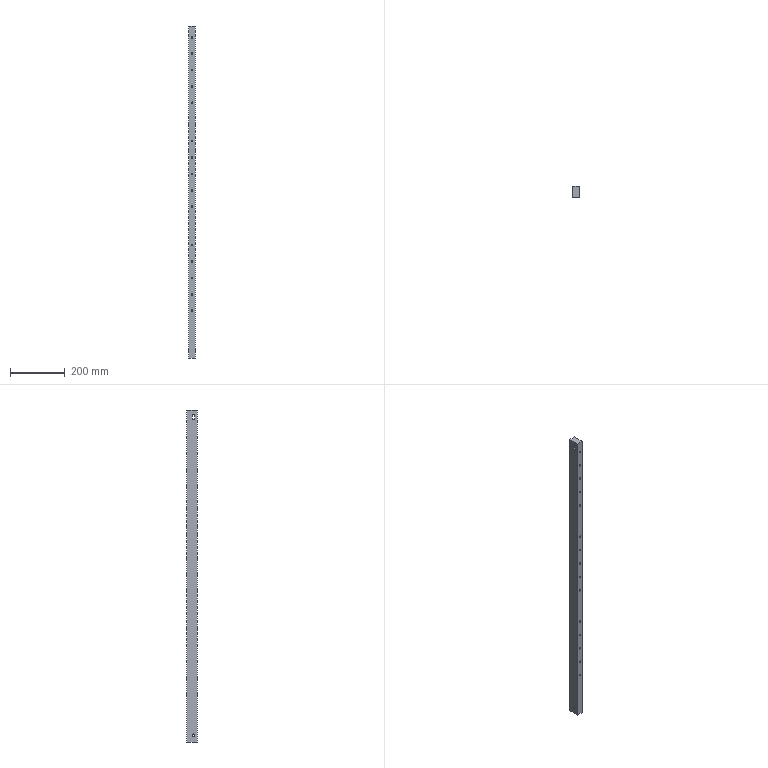Part | STEP file | 750038351 | 1 solid | 43 faces | box 25 x 40 x 1214 mm | volume 1190455 mm3 | cylinder 35 | plane 8 | commonest cylinder face diameters 6.2 x30 9 x5
STEP:
#1=CARTESIAN_POINT('',(-12.5,15.,1179.5));
#2=VERTEX_POINT('',#1);
#3=CARTESIAN_POINT('',(-12.5,19.5,1184.));
#4=VERTEX_POINT('',#3);
#5=CARTESIAN_POINT('',(-12.5,15.,1184.));
#6=DIRECTION('',(1.,0.,0.));
#7=DIRECTION('',(0.,0.,-1.));
#8=AXIS2_PLACEMENT_3D('',#5,#6,#7);
#9=CIRCLE('',#8,4.5);
#10=EDGE_CURVE('',#2,#4,#9,.T.);
#11=ORIENTED_EDGE('',*,*,#10,.F.);
#12=CARTESIAN_POINT('',(12.5,15.,1179.5));
#13=VERTEX_POINT('',#12);
#14=CARTESIAN_POINT('',(-15.,15.,1179.5));
#15=DIRECTION('',(1.,0.,0.));
#16=VECTOR('',#15,1000.);
#17=LINE('',#14,#16);
#18=EDGE_CURVE('',#2,#13,#17,.T.);
#19=ORIENTED_EDGE('',*,*,#18,.T.);
#20=CARTESIAN_POINT('',(12.5,19.5,1184.));
#21=VERTEX_POINT('',#20);
#22=CARTESIAN_POINT('',(12.5,15.,1184.));
#23=DIRECTION('',(1.,0.,0.));
#24=DIRECTION('',(0.,0.,-1.));
#25=AXIS2_PLACEMENT_3D('',#22,#23,#24);
#26=CIRCLE('',#25,4.5);
#27=EDGE_CURVE('',#13,#21,#26,.T.);
#28=ORIENTED_EDGE('',*,*,#27,.T.);
#29=CARTESIAN_POINT('',(-15.,19.5,1184.));
#30=DIRECTION('',(-1.,0.,0.));
#31=VECTOR('',#30,1000.);
#32=LINE('',#29,#31);
#33=EDGE_CURVE('',#21,#4,#32,.T.);
#34=ORIENTED_EDGE('',*,*,#33,.T.);
#35=EDGE_LOOP('',(#11,#19,#28,#34));
#36=FACE_OUTER_BOUND('',#35,.T.);
#37=CARTESIAN_POINT('',(-15.,15.,1184.));
#38=DIRECTION('',(1.,0.,0.));
#39=DIRECTION('',(0.,0.,-1.));
#40=AXIS2_PLACEMENT_3D('',#37,#38,#39);
#41=CYLINDRICAL_SURFACE('',#40,4.5);
#42=ADVANCED_FACE('',(#36),#41,.F.);
#43=CARTESIAN_POINT('',(-12.5,15.,29.5));
#44=VERTEX_POINT('',#43);
#45=CARTESIAN_POINT('',(-12.5,15.,20.5));
#46=VERTEX_POINT('',#45);
#47=CARTESIAN_POINT('',(-12.5,15.,25.));
#48=DIRECTION('',(1.,0.,0.));
#49=DIRECTION('',(0.,0.,-1.));
#50=AXIS2_PLACEMENT_3D('',#47,#48,#49);
#51=CIRCLE('',#50,4.5);
#52=EDGE_CURVE('',#44,#46,#51,.T.);
#53=ORIENTED_EDGE('',*,*,#52,.F.);
#54=CARTESIAN_POINT('',(12.5,15.,29.5));
#55=VERTEX_POINT('',#54);
#56=CARTESIAN_POINT('',(-15.,15.,29.5));
#57=DIRECTION('',(1.,0.,0.));
#58=VECTOR('',#57,1000.);
#59=LINE('',#56,#58);
#60=EDGE_CURVE('',#44,#55,#59,.T.);
#61=ORIENTED_EDGE('',*,*,#60,.T.);
#62=CARTESIAN_POINT('',(12.5,15.,20.5));
#63=VERTEX_POINT('',#62);
#64=CARTESIAN_POINT('',(12.5,15.,25.));
#65=DIRECTION('',(1.,0.,0.));
#66=DIRECTION('',(0.,0.,-1.));
#67=AXIS2_PLACEMENT_3D('',#64,#65,#66);
#68=CIRCLE('',#67,4.5);
#69=EDGE_CURVE('',#55,#63,#68,.T.);
#70=ORIENTED_EDGE('',*,*,#69,.T.);
#71=CARTESIAN_POINT('',(-15.,15.,20.5));
#72=DIRECTION('',(1.,0.,0.));
#73=VECTOR('',#72,1000.);
#74=LINE('',#71,#73);
#75=EDGE_CURVE('',#46,#63,#74,.T.);
#76=ORIENTED_EDGE('',*,*,#75,.F.);
#77=EDGE_LOOP('',(#53,#61,#70,#76));
#78=FACE_OUTER_BOUND('',#77,.T.);
#79=CARTESIAN_POINT('',(-15.,15.,25.));
#80=DIRECTION('',(1.,0.,0.));
#81=DIRECTION('',(0.,0.,-1.));
#82=AXIS2_PLACEMENT_3D('',#79,#80,#81);
#83=CYLINDRICAL_SURFACE('',#82,4.5);
#84=ADVANCED_FACE('',(#78),#83,.F.);
#85=CARTESIAN_POINT('',(0.000000003,40.,1109.9));
#86=VERTEX_POINT('',#85);
#87=CARTESIAN_POINT('',(0.000000003,40.,1116.1));
#88=VERTEX_POINT('',#87);
#89=CARTESIAN_POINT('',(0.000000003,40.,1113.));
#90=DIRECTION('',(0.,1.,0.));
#91=DIRECTION('',(0.,0.,-1.));
#92=AXIS2_PLACEMENT_3D('',#89,#90,#91);
#93=CIRCLE('',#92,3.1);
#94=EDGE_CURVE('',#86,#88,#93,.T.);
#95=ORIENTED_EDGE('',*,*,#94,.T.);
#96=CARTESIAN_POINT('',(0.000000003,0.,1116.1));
#97=VERTEX_POINT('',#96);
#98=CARTESIAN_POINT('',(0.000000003,44.,1116.1));
#99=DIRECTION('',(0.,-1.,0.));
#100=VECTOR('',#99,1000.);
#101=LINE('',#98,#100);
#102=EDGE_CURVE('',#88,#97,#101,.T.);
#103=ORIENTED_EDGE('',*,*,#102,.T.);
#104=CARTESIAN_POINT('',(0.000000003,0.,1109.9));
#105=VERTEX_POINT('',#104);
#106=CARTESIAN_POINT('',(0.000000003,0.,1113.));
#107=DIRECTION('',(0.,-1.,0.));
#108=DIRECTION('',(0.,0.,-1.));
#109=AXIS2_PLACEMENT_3D('',#106,#107,#108);
#110=CIRCLE('',#109,3.1);
#111=EDGE_CURVE('',#97,#105,#110,.T.);
#112=ORIENTED_EDGE('',*,*,#111,.T.);
#113=CARTESIAN_POINT('',(0.000000003,44.,1109.9));
#114=DIRECTION('',(0.,-1.,0.));
#115=VECTOR('',#114,1000.);
#116=LINE('',#113,#115);
#117=EDGE_CURVE('',#86,#105,#116,.T.);
#118=ORIENTED_EDGE('',*,*,#117,.F.);
#119=EDGE_LOOP('',(#95,#103,#112,#118));
#120=FACE_OUTER_BOUND('',#119,.T.);
#121=CARTESIAN_POINT('',(0.000000003,44.,1113.));
#122=DIRECTION('',(0.,-1.,0.));
#123=DIRECTION('',(0.,0.,-1.));
#124=AXIS2_PLACEMENT_3D('',#121,#122,#123);
#125=CYLINDRICAL_SURFACE('',#124,3.1);
#126=ADVANCED_FACE('',(#120),#125,.F.);
#127=CARTESIAN_POINT('',(0.000000003,40.,1169.9));
#128=VERTEX_POINT('',#127);
#129=CARTESIAN_POINT('',(0.000000003,40.,1176.1));
#130=VERTEX_POINT('',#129);
#131=CARTESIAN_POINT('',(0.000000003,40.,1173.));
#132=DIRECTION('',(0.,1.,0.));
#133=DIRECTION('',(0.,0.,-1.));
#134=AXIS2_PLACEMENT_3D('',#131,#132,#133);
#135=CIRCLE('',#134,3.1);
#136=EDGE_CURVE('',#128,#130,#135,.T.);
#137=ORIENTED_EDGE('',*,*,#136,.T.);
#138=CARTESIAN_POINT('',(0.000000003,0.,1176.1));
#139=VERTEX_POINT('',#138);
#140=CARTESIAN_POINT('',(0.000000003,44.,1176.1));
#141=DIRECTION('',(0.,-1.,0.));
#142=VECTOR('',#141,1000.);
#143=LINE('',#140,#142);
#144=EDGE_CURVE('',#130,#139,#143,.T.);
#145=ORIENTED_EDGE('',*,*,#144,.T.);
#146=CARTESIAN_POINT('',(0.000000003,0.,1169.9));
#147=VERTEX_POINT('',#146);
#148=CARTESIAN_POINT('',(0.000000003,0.,1173.));
#149=DIRECTION('',(0.,-1.,0.));
#150=DIRECTION('',(0.,0.,-1.));
#151=AXIS2_PLACEMENT_3D('',#148,#149,#150);
#152=CIRCLE('',#151,3.1);
#153=EDGE_CURVE('',#139,#147,#152,.T.);
#154=ORIENTED_EDGE('',*,*,#153,.T.);
#155=CARTESIAN_POINT('',(0.000000003,44.,1169.9));
#156=DIRECTION('',(0.,-1.,0.));
#157=VECTOR('',#156,1000.);
#158=LINE('',#155,#157);
#159=EDGE_CURVE('',#128,#147,#158,.T.);
#160=ORIENTED_EDGE('',*,*,#159,.F.);
#161=EDGE_LOOP('',(#137,#145,#154,#160));
#162=FACE_OUTER_BOUND('',#161,.T.);
#163=CARTESIAN_POINT('',(0.000000003,44.,1173.));
#164=DIRECTION('',(0.,-1.,0.));
#165=DIRECTION('',(0.,0.,-1.));
#166=AXIS2_PLACEMENT_3D('',#163,#164,#165);
#167=CYLINDRICAL_SURFACE('',#166,3.1);
#168=ADVANCED_FACE('',(#162),#167,.F.);
#169=CARTESIAN_POINT('',(0.000000003,40.,1049.9));
#170=VERTEX_POINT('',#169);
#171=CARTESIAN_POINT('',(0.000000003,40.,1056.1));
#172=VERTEX_POINT('',#171);
#173=CARTESIAN_POINT('',(0.000000003,40.,1053.));
#174=DIRECTION('',(0.,1.,0.));
#175=DIRECTION('',(0.,0.,-1.));
#176=AXIS2_PLACEMENT_3D('',#173,#174,#175);
#177=CIRCLE('',#176,3.1);
#178=EDGE_CURVE('',#170,#172,#177,.T.);
#179=ORIENTED_EDGE('',*,*,#178,.T.);
#180=CARTESIAN_POINT('',(0.000000003,0.,1056.1));
#181=VERTEX_POINT('',#180);
#182=CARTESIAN_POINT('',(0.000000003,44.,1056.1));
#183=DIRECTION('',(0.,-1.,0.));
#184=VECTOR('',#183,1000.);
#185=LINE('',#182,#184);
#186=EDGE_CURVE('',#172,#181,#185,.T.);
#187=ORIENTED_EDGE('',*,*,#186,.T.);
#188=CARTESIAN_POINT('',(0.000000003,0.,1049.9));
#189=VERTEX_POINT('',#188);
#190=CARTESIAN_POINT('',(0.000000003,0.,1053.));
#191=DIRECTION('',(0.,-1.,0.));
#192=DIRECTION('',(0.,0.,-1.));
#193=AXIS2_PLACEMENT_3D('',#190,#191,#192);
#194=CIRCLE('',#193,3.1);
#195=EDGE_CURVE('',#181,#189,#194,.T.);
#196=ORIENTED_EDGE('',*,*,#195,.T.);
#197=CARTESIAN_POINT('',(0.000000003,44.,1049.9));
#198=DIRECTION('',(0.,-1.,0.));
#199=VECTOR('',#198,1000.);
#200=LINE('',#197,#199);
#201=EDGE_CURVE('',#170,#189,#200,.T.);
#202=ORIENTED_EDGE('',*,*,#201,.F.);
#203=EDGE_LOOP('',(#179,#187,#196,#202));
#204=FACE_OUTER_BOUND('',#203,.T.);
#205=CARTESIAN_POINT('',(0.000000003,44.,1053.));
#206=DIRECTION('',(0.,-1.,0.));
#207=DIRECTION('',(0.,0.,-1.));
#208=AXIS2_PLACEMENT_3D('',#205,#206,#207);
#209=CYLINDRICAL_SURFACE('',#208,3.1);
#210=ADVANCED_FACE('',(#204),#209,.F.);
#211=CARTESIAN_POINT('',(0.000000003,40.,929.9));
#212=VERTEX_POINT('',#211);
#213=CARTESIAN_POINT('',(0.000000003,40.,936.1));
#214=VERTEX_POINT('',#213);
#215=CARTESIAN_POINT('',(0.000000003,40.,933.));
#216=DIRECTION('',(0.,1.,0.));
#217=DIRECTION('',(0.,0.,-1.));
#218=AXIS2_PLACEMENT_3D('',#215,#216,#217);
#219=CIRCLE('',#218,3.1);
#220=EDGE_CURVE('',#212,#214,#219,.T.);
#221=ORIENTED_EDGE('',*,*,#220,.T.);
#222=CARTESIAN_POINT('',(0.000000003,0.,936.1));
#223=VERTEX_POINT('',#222);
#224=CARTESIAN_POINT('',(0.000000003,44.,936.1));
#225=DIRECTION('',(0.,-1.,0.));
#226=VECTOR('',#225,1000.);
#227=LINE('',#224,#226);
#228=EDGE_CURVE('',#214,#223,#227,.T.);
#229=ORIENTED_EDGE('',*,*,#228,.T.);
#230=CARTESIAN_POINT('',(0.000000003,0.,929.9));
#231=VERTEX_POINT('',#230);
#232=CARTESIAN_POINT('',(0.000000003,0.,933.));
#233=DIRECTION('',(0.,-1.,0.));
#234=DIRECTION('',(0.,0.,-1.));
#235=AXIS2_PLACEMENT_3D('',#232,#233,#234);
#236=CIRCLE('',#235,3.1);
#237=EDGE_CURVE('',#223,#231,#236,.T.);
#238=ORIENTED_EDGE('',*,*,#237,.T.);
#239=CARTESIAN_POINT('',(0.000000003,44.,929.9));
#240=DIRECTION('',(0.,-1.,0.));
#241=VECTOR('',#240,1000.);
#242=LINE('',#239,#241);
#243=EDGE_CURVE('',#212,#231,#242,.T.);
#244=ORIENTED_EDGE('',*,*,#243,.F.);
#245=EDGE_LOOP('',(#221,#229,#238,#244));
#246=FACE_OUTER_BOUND('',#245,.T.);
#247=CARTESIAN_POINT('',(0.000000003,44.,933.));
#248=DIRECTION('',(0.,-1.,0.));
#249=DIRECTION('',(0.,0.,-1.));
#250=AXIS2_PLACEMENT_3D('',#247,#248,#249);
#251=CYLINDRICAL_SURFACE('',#250,3.1);
#252=ADVANCED_FACE('',(#246),#251,.F.);
#253=CARTESIAN_POINT('',(0.000000003,40.,729.9));
#254=VERTEX_POINT('',#253);
#255=CARTESIAN_POINT('',(0.000000003,40.,736.1));
#256=VERTEX_POINT('',#255);
#257=CARTESIAN_POINT('',(0.000000003,40.,733.));
#258=DIRECTION('',(0.,1.,0.));
#259=DIRECTION('',(0.,0.,-1.));
#260=AXIS2_PLACEMENT_3D('',#257,#258,#259);
#261=CIRCLE('',#260,3.1);
#262=EDGE_CURVE('',#254,#256,#261,.T.);
#263=ORIENTED_EDGE('',*,*,#262,.T.);
#264=CARTESIAN_POINT('',(0.000000003,0.,736.1));
#265=VERTEX_POINT('',#264);
#266=CARTESIAN_POINT('',(0.000000003,44.,736.1));
#267=DIRECTION('',(0.,-1.,0.));
#268=VECTOR('',#267,1000.);
#269=LINE('',#266,#268);
#270=EDGE_CURVE('',#256,#265,#269,.T.);
#271=ORIENTED_EDGE('',*,*,#270,.T.);
#272=CARTESIAN_POINT('',(0.000000003,0.,729.9));
#273=VERTEX_POINT('',#272);
#274=CARTESIAN_POINT('',(0.000000003,0.,733.));
#275=DIRECTION('',(0.,-1.,0.));
#276=DIRECTION('',(0.,0.,-1.));
#277=AXIS2_PLACEMENT_3D('',#274,#275,#276);
#278=CIRCLE('',#277,3.1);
#279=EDGE_CURVE('',#265,#273,#278,.T.);
#280=ORIENTED_EDGE('',*,*,#279,.T.);
#281=CARTESIAN_POINT('',(0.000000003,44.,729.9));
#282=DIRECTION('',(0.,-1.,0.));
#283=VECTOR('',#282,1000.);
#284=LINE('',#281,#283);
#285=EDGE_CURVE('',#254,#273,#284,.T.);
#286=ORIENTED_EDGE('',*,*,#285,.F.);
#287=EDGE_LOOP('',(#263,#271,#280,#286));
#288=FACE_OUTER_BOUND('',#287,.T.);
#289=CARTESIAN_POINT('',(0.000000003,44.,733.));
#290=DIRECTION('',(0.,-1.,0.));
#291=DIRECTION('',(0.,0.,-1.));
#292=AXIS2_PLACEMENT_3D('',#289,#290,#291);
#293=CYLINDRICAL_SURFACE('',#292,3.1);
#294=ADVANCED_FACE('',(#288),#293,.F.);
#295=CARTESIAN_POINT('',(0.000000003,40.,609.9));
#296=VERTEX_POINT('',#295);
#297=CARTESIAN_POINT('',(0.000000003,40.,616.1));
#298=VERTEX_POINT('',#297);
#299=CARTESIAN_POINT('',(0.000000003,40.,613.));
#300=DIRECTION('',(0.,1.,0.));
#301=DIRECTION('',(0.,0.,-1.));
#302=AXIS2_PLACEMENT_3D('',#299,#300,#301);
#303=CIRCLE('',#302,3.1);
#304=EDGE_CURVE('',#296,#298,#303,.T.);
#305=ORIENTED_EDGE('',*,*,#304,.T.);
#306=CARTESIAN_POINT('',(0.000000003,0.,616.1));
#307=VERTEX_POINT('',#306);
#308=CARTESIAN_POINT('',(0.000000003,44.,616.1));
#309=DIRECTION('',(0.,-1.,0.));
#310=VECTOR('',#309,1000.);
#311=LINE('',#308,#310);
#312=EDGE_CURVE('',#298,#307,#311,.T.);
#313=ORIENTED_EDGE('',*,*,#312,.T.);
#314=CARTESIAN_POINT('',(0.000000003,0.,609.9));
#315=VERTEX_POINT('',#314);
#316=CARTESIAN_POINT('',(0.000000003,0.,613.));
#317=DIRECTION('',(0.,-1.,0.));
#318=DIRECTION('',(0.,0.,-1.));
#319=AXIS2_PLACEMENT_3D('',#316,#317,#318);
#320=CIRCLE('',#319,3.1);
#321=EDGE_CURVE('',#307,#315,#320,.T.);
#322=ORIENTED_EDGE('',*,*,#321,.T.);
#323=CARTESIAN_POINT('',(0.000000003,44.,609.9));
#324=DIRECTION('',(0.,-1.,0.));
#325=VECTOR('',#324,1000.);
#326=LINE('',#323,#325);
#327=EDGE_CURVE('',#296,#315,#326,.T.);
#328=ORIENTED_EDGE('',*,*,#327,.F.);
#329=EDGE_LOOP('',(#305,#313,#322,#328));
#330=FACE_OUTER_BOUND('',#329,.T.);
#331=CARTESIAN_POINT('',(0.000000003,44.,613.));
#332=DIRECTION('',(0.,-1.,0.));
#333=DIRECTION('',(0.,0.,-1.));
#334=AXIS2_PLACEMENT_3D('',#331,#332,#333);
#335=CYLINDRICAL_SURFACE('',#334,3.1);
#336=ADVANCED_FACE('',(#330),#335,.F.);
#337=CARTESIAN_POINT('',(0.000000003,40.,409.9));
#338=VERTEX_POINT('',#337);
#339=CARTESIAN_POINT('',(0.000000003,40.,416.1));
#340=VERTEX_POINT('',#339);
#341=CARTESIAN_POINT('',(0.000000003,40.,413.));
#342=DIRECTION('',(0.,1.,0.));
#343=DIRECTION('',(0.,0.,-1.));
#344=AXIS2_PLACEMENT_3D('',#341,#342,#343);
#345=CIRCLE('',#344,3.1);
#346=EDGE_CURVE('',#338,#340,#345,.T.);
#347=ORIENTED_EDGE('',*,*,#346,.T.);
#348=CARTESIAN_POINT('',(0.000000003,0.,416.1));
#349=VERTEX_POINT('',#348);
#350=CARTESIAN_POINT('',(0.000000003,44.,416.1));
#351=DIRECTION('',(0.,-1.,0.));
#352=VECTOR('',#351,1000.);
#353=LINE('',#350,#352);
#354=EDGE_CURVE('',#340,#349,#353,.T.);
#355=ORIENTED_EDGE('',*,*,#354,.T.);
#356=CARTESIAN_POINT('',(0.000000003,0.,409.9));
#357=VERTEX_POINT('',#356);
#358=CARTESIAN_POINT('',(0.000000003,0.,413.));
#359=DIRECTION('',(0.,-1.,0.));
#360=DIRECTION('',(0.,0.,-1.));
#361=AXIS2_PLACEMENT_3D('',#358,#359,#360);
#362=CIRCLE('',#361,3.1);
#363=EDGE_CURVE('',#349,#357,#362,.T.);
#364=ORIENTED_EDGE('',*,*,#363,.T.);
#365=CARTESIAN_POINT('',(0.000000003,44.,409.9));
#366=DIRECTION('',(0.,-1.,0.));
#367=VECTOR('',#366,1000.);
#368=LINE('',#365,#367);
#369=EDGE_CURVE('',#338,#357,#368,.T.);
#370=ORIENTED_EDGE('',*,*,#369,.F.);
#371=EDGE_LOOP('',(#347,#355,#364,#370));
#372=FACE_OUTER_BOUND('',#371,.T.);
#373=CARTESIAN_POINT('',(0.000000003,44.,413.));
#374=DIRECTION('',(0.,-1.,0.));
#375=DIRECTION('',(0.,0.,-1.));
#376=AXIS2_PLACEMENT_3D('',#373,#374,#375);
#377=CYLINDRICAL_SURFACE('',#376,3.1);
#378=ADVANCED_FACE('',(#372),#377,.F.);
#379=CARTESIAN_POINT('',(0.000000003,40.,349.9));
#380=VERTEX_POINT('',#379);
#381=CARTESIAN_POINT('',(0.000000003,40.,356.1));
#382=VERTEX_POINT('',#381);
#383=CARTESIAN_POINT('',(0.000000003,40.,353.));
#384=DIRECTION('',(0.,1.,0.));
#385=DIRECTION('',(0.,0.,-1.));
#386=AXIS2_PLACEMENT_3D('',#383,#384,#385);
#387=CIRCLE('',#386,3.1);
#388=EDGE_CURVE('',#380,#382,#387,.T.);
#389=ORIENTED_EDGE('',*,*,#388,.T.);
#390=CARTESIAN_POINT('',(0.000000003,0.,356.1));
#391=VERTEX_POINT('',#390);
#392=CARTESIAN_POINT('',(0.000000003,44.,356.1));
#393=DIRECTION('',(0.,-1.,0.));
#394=VECTOR('',#393,1000.);
#395=LINE('',#392,#394);
#396=EDGE_CURVE('',#382,#391,#395,.T.);
#397=ORIENTED_EDGE('',*,*,#396,.T.);
#398=CARTESIAN_POINT('',(0.000000003,0.,349.9));
#399=VERTEX_POINT('',#398);
#400=CARTESIAN_POINT('',(0.000000003,0.,353.));
#401=DIRECTION('',(0.,-1.,0.));
#402=DIRECTION('',(0.,0.,-1.));
#403=AXIS2_PLACEMENT_3D('',#400,#401,#402);
#404=CIRCLE('',#403,3.1);
#405=EDGE_CURVE('',#391,#399,#404,.T.);
#406=ORIENTED_EDGE('',*,*,#405,.T.);
#407=CARTESIAN_POINT('',(0.000000003,44.,349.9));
#408=DIRECTION('',(0.,-1.,0.));
#409=VECTOR('',#408,1000.);
#410=LINE('',#407,#409);
#411=EDGE_CURVE('',#380,#399,#410,.T.);
#412=ORIENTED_EDGE('',*,*,#411,.F.);
#413=EDGE_LOOP('',(#389,#397,#406,#412));
#414=FACE_OUTER_BOUND('',#413,.T.);
#415=CARTESIAN_POINT('',(0.000000003,44.,353.));
#416=DIRECTION('',(0.,-1.,0.));
#417=DIRECTION('',(0.,0.,-1.));
#418=AXIS2_PLACEMENT_3D('',#415,#416,#417);
#419=CYLINDRICAL_SURFACE('',#418,3.1);
#420=ADVANCED_FACE('',(#414),#419,.F.);
#421=CARTESIAN_POINT('',(0.000000003,40.,229.9));
#422=VERTEX_POINT('',#421);
#423=CARTESIAN_POINT('',(0.000000003,40.,236.1));
#424=VERTEX_POINT('',#423);
#425=CARTESIAN_POINT('',(0.000000003,40.,233.));
#426=DIRECTION('',(0.,1.,0.));
#427=DIRECTION('',(0.,0.,-1.));
#428=AXIS2_PLACEMENT_3D('',#425,#426,#427);
#429=CIRCLE('',#428,3.1);
#430=EDGE_CURVE('',#422,#424,#429,.T.);
#431=ORIENTED_EDGE('',*,*,#430,.T.);
#432=CARTESIAN_POINT('',(0.000000003,0.,236.1));
#433=VERTEX_POINT('',#432);
#434=CARTESIAN_POINT('',(0.000000003,44.,236.1));
#435=DIRECTION('',(0.,-1.,0.));
#436=VECTOR('',#435,1000.);
#437=LINE('',#434,#436);
#438=EDGE_CURVE('',#424,#433,#437,.T.);
#439=ORIENTED_EDGE('',*,*,#438,.T.);
#440=CARTESIAN_POINT('',(0.000000003,0.,229.9));
#441=VERTEX_POINT('',#440);
#442=CARTESIAN_POINT('',(0.000000003,0.,233.));
#443=DIRECTION('',(0.,-1.,0.));
#444=DIRECTION('',(0.,0.,-1.));
#445=AXIS2_PLACEMENT_3D('',#442,#443,#444);
#446=CIRCLE('',#445,3.1);
#447=EDGE_CURVE('',#433,#441,#446,.T.);
#448=ORIENTED_EDGE('',*,*,#447,.T.);
#449=CARTESIAN_POINT('',(0.000000003,44.,229.9));
#450=DIRECTION('',(0.,-1.,0.));
#451=VECTOR('',#450,1000.);
#452=LINE('',#449,#451);
#453=EDGE_CURVE('',#422,#441,#452,.T.);
#454=ORIENTED_EDGE('',*,*,#453,.F.);
#455=EDGE_LOOP('',(#431,#439,#448,#454));
#456=FACE_OUTER_BOUND('',#455,.T.);
#457=CARTESIAN_POINT('',(0.000000003,44.,233.));
#458=DIRECTION('',(0.,-1.,0.));
#459=DIRECTION('',(0.,0.,-1.));
#460=AXIS2_PLACEMENT_3D('',#457,#458,#459);
#461=CYLINDRICAL_SURFACE('',#460,3.1);
#462=ADVANCED_FACE('',(#456),#461,.F.);
#463=CARTESIAN_POINT('',(0.000000003,40.,169.9));
#464=VERTEX_POINT('',#463);
#465=CARTESIAN_POINT('',(0.000000003,40.,176.1));
#466=VERTEX_POINT('',#465);
#467=CARTESIAN_POINT('',(0.000000003,40.,173.));
#468=DIRECTION('',(0.,1.,0.));
#469=DIRECTION('',(0.,0.,-1.));
#470=AXIS2_PLACEMENT_3D('',#467,#468,#469);
#471=CIRCLE('',#470,3.1);
#472=EDGE_CURVE('',#464,#466,#471,.T.);
#473=ORIENTED_EDGE('',*,*,#472,.T.);
#474=CARTESIAN_POINT('',(0.000000003,0.,176.1));
#475=VERTEX_POINT('',#474);
#476=CARTESIAN_POINT('',(0.000000003,44.,176.1));
#477=DIRECTION('',(0.,-1.,0.));
#478=VECTOR('',#477,1000.);
#479=LINE('',#476,#478);
#480=EDGE_CURVE('',#466,#475,#479,.T.);
#481=ORIENTED_EDGE('',*,*,#480,.T.);
#482=CARTESIAN_POINT('',(0.000000003,0.,169.9));
#483=VERTEX_POINT('',#482);
#484=CARTESIAN_POINT('',(0.000000003,0.,173.));
#485=DIRECTION('',(0.,-1.,0.));
#486=DIRECTION('',(0.,0.,-1.));
#487=AXIS2_PLACEMENT_3D('',#484,#485,#486);
#488=CIRCLE('',#487,3.1);
#489=EDGE_CURVE('',#475,#483,#488,.T.);
#490=ORIENTED_EDGE('',*,*,#489,.T.);
#491=CARTESIAN_POINT('',(0.000000003,44.,169.9));
#492=DIRECTION('',(0.,-1.,0.));
#493=VECTOR('',#492,1000.);
#494=LINE('',#491,#493);
#495=EDGE_CURVE('',#464,#483,#494,.T.);
#496=ORIENTED_EDGE('',*,*,#495,.F.);
#497=EDGE_LOOP('',(#473,#481,#490,#496));
#498=FACE_OUTER_BOUND('',#497,.T.);
#499=CARTESIAN_POINT('',(0.000000003,44.,173.));
#500=DIRECTION('',(0.,-1.,0.));
#501=DIRECTION('',(0.,0.,-1.));
#502=AXIS2_PLACEMENT_3D('',#499,#500,#501);
#503=CYLINDRICAL_SURFACE('',#502,3.1);
#504=ADVANCED_FACE('',(#498),#503,.F.);
#505=CARTESIAN_POINT('',(0.000000003,40.,289.9));
#506=VERTEX_POINT('',#505);
#507=CARTESIAN_POINT('',(0.000000003,40.,296.1));
#508=VERTEX_POINT('',#507);
#509=CARTESIAN_POINT('',(0.000000003,40.,293.));
#510=DIRECTION('',(0.,1.,0.));
#511=DIRECTION('',(0.,0.,-1.));
#512=AXIS2_PLACEMENT_3D('',#509,#510,#511);
#513=CIRCLE('',#512,3.1);
#514=EDGE_CURVE('',#506,#508,#513,.T.);
#515=ORIENTED_EDGE('',*,*,#514,.T.);
#516=CARTESIAN_POINT('',(0.000000003,0.,296.1));
#517=VERTEX_POINT('',#516);
#518=CARTESIAN_POINT('',(0.000000003,44.,296.1));
#519=DIRECTION('',(0.,-1.,0.));
#520=VECTOR('',#519,1000.);
#521=LINE('',#518,#520);
#522=EDGE_CURVE('',#508,#517,#521,.T.);
#523=ORIENTED_EDGE('',*,*,#522,.T.);
#524=CARTESIAN_POINT('',(0.000000003,0.,289.9));
#525=VERTEX_POINT('',#524);
#526=CARTESIAN_POINT('',(0.000000003,0.,293.));
#527=DIRECTION('',(0.,-1.,0.));
#528=DIRECTION('',(0.,0.,-1.));
#529=AXIS2_PLACEMENT_3D('',#526,#527,#528);
#530=CIRCLE('',#529,3.1);
#531=EDGE_CURVE('',#517,#525,#530,.T.);
#532=ORIENTED_EDGE('',*,*,#531,.T.);
#533=CARTESIAN_POINT('',(0.000000003,44.,289.9));
#534=DIRECTION('',(0.,-1.,0.));
#535=VECTOR('',#534,1000.);
#536=LINE('',#533,#535);
#537=EDGE_CURVE('',#506,#525,#536,.T.);
#538=ORIENTED_EDGE('',*,*,#537,.F.);
#539=EDGE_LOOP('',(#515,#523,#532,#538));
#540=FACE_OUTER_BOUND('',#539,.T.);
#541=CARTESIAN_POINT('',(0.000000003,44.,293.));
#542=DIRECTION('',(0.,-1.,0.));
#543=DIRECTION('',(0.,0.,-1.));
#544=AXIS2_PLACEMENT_3D('',#541,#542,#543);
#545=CYLINDRICAL_SURFACE('',#544,3.1);
#546=ADVANCED_FACE('',(#540),#545,.F.);
#547=CARTESIAN_POINT('',(0.000000003,40.,549.9));
#548=VERTEX_POINT('',#547);
#549=CARTESIAN_POINT('',(0.000000003,40.,556.1));
#550=VERTEX_POINT('',#549);
#551=CARTESIAN_POINT('',(0.000000003,40.,553.));
#552=DIRECTION('',(0.,1.,0.));
#553=DIRECTION('',(0.,0.,-1.));
#554=AXIS2_PLACEMENT_3D('',#551,#552,#553);
#555=CIRCLE('',#554,3.1);
#556=EDGE_CURVE('',#548,#550,#555,.T.);
#557=ORIENTED_EDGE('',*,*,#556,.T.);
#558=CARTESIAN_POINT('',(0.000000003,0.,556.1));
#559=VERTEX_POINT('',#558);
#560=CARTESIAN_POINT('',(0.000000003,44.,556.1));
#561=DIRECTION('',(0.,-1.,0.));
#562=VECTOR('',#561,1000.);
#563=LINE('',#560,#562);
#564=EDGE_CURVE('',#550,#559,#563,.T.);
#565=ORIENTED_EDGE('',*,*,#564,.T.);
#566=CARTESIAN_POINT('',(0.000000003,0.,549.9));
#567=VERTEX_POINT('',#566);
#568=CARTESIAN_POINT('',(0.000000003,0.,553.));
#569=DIRECTION('',(0.,-1.,0.));
#570=DIRECTION('',(0.,0.,-1.));
#571=AXIS2_PLACEMENT_3D('',#568,#569,#570);
#572=CIRCLE('',#571,3.1);
#573=EDGE_CURVE('',#559,#567,#572,.T.);
#574=ORIENTED_EDGE('',*,*,#573,.T.);
#575=CARTESIAN_POINT('',(0.000000003,44.,549.9));
#576=DIRECTION('',(0.,-1.,0.));
#577=VECTOR('',#576,1000.);
#578=LINE('',#575,#577);
#579=EDGE_CURVE('',#548,#567,#578,.T.);
#580=ORIENTED_EDGE('',*,*,#579,.F.);
#581=EDGE_LOOP('',(#557,#565,#574,#580));
#582=FACE_OUTER_BOUND('',#581,.T.);
#583=CARTESIAN_POINT('',(0.000000003,44.,553.));
#584=DIRECTION('',(0.,-1.,0.));
#585=DIRECTION('',(0.,0.,-1.));
#586=AXIS2_PLACEMENT_3D('',#583,#584,#585);
#587=CYLINDRICAL_SURFACE('',#586,3.1);
#588=ADVANCED_FACE('',(#582),#587,.F.);
#589=CARTESIAN_POINT('',(0.000000003,40.,669.9));
#590=VERTEX_POINT('',#589);
#591=CARTESIAN_POINT('',(0.000000003,40.,676.1));
#592=VERTEX_POINT('',#591);
#593=CARTESIAN_POINT('',(0.000000003,40.,673.));
#594=DIRECTION('',(0.,1.,0.));
#595=DIRECTION('',(0.,0.,-1.));
#596=AXIS2_PLACEMENT_3D('',#593,#594,#595);
#597=CIRCLE('',#596,3.1);
#598=EDGE_CURVE('',#590,#592,#597,.T.);
#599=ORIENTED_EDGE('',*,*,#598,.T.);
#600=CARTESIAN_POINT('',(0.000000003,0.,676.1));
#601=VERTEX_POINT('',#600);
#602=CARTESIAN_POINT('',(0.000000003,44.,676.1));
#603=DIRECTION('',(0.,-1.,0.));
#604=VECTOR('',#603,1000.);
#605=LINE('',#602,#604);
#606=EDGE_CURVE('',#592,#601,#605,.T.);
#607=ORIENTED_EDGE('',*,*,#606,.T.);
#608=CARTESIAN_POINT('',(0.000000003,0.,669.9));
#609=VERTEX_POINT('',#608);
#610=CARTESIAN_POINT('',(0.000000003,0.,673.));
#611=DIRECTION('',(0.,-1.,0.));
#612=DIRECTION('',(0.,0.,-1.));
#613=AXIS2_PLACEMENT_3D('',#610,#611,#612);
#614=CIRCLE('',#613,3.1);
#615=EDGE_CURVE('',#601,#609,#614,.T.);
#616=ORIENTED_EDGE('',*,*,#615,.T.);
#617=CARTESIAN_POINT('',(0.000000003,44.,669.9));
#618=DIRECTION('',(0.,-1.,0.));
#619=VECTOR('',#618,1000.);
#620=LINE('',#617,#619);
#621=EDGE_CURVE('',#590,#609,#620,.T.);
#622=ORIENTED_EDGE('',*,*,#621,.F.);
#623=EDGE_LOOP('',(#599,#607,#616,#622));
#624=FACE_OUTER_BOUND('',#623,.T.);
#625=CARTESIAN_POINT('',(0.000000003,44.,673.));
#626=DIRECTION('',(0.,-1.,0.));
#627=DIRECTION('',(0.,0.,-1.));
#628=AXIS2_PLACEMENT_3D('',#625,#626,#627);
#629=CYLINDRICAL_SURFACE('',#628,3.1);
#630=ADVANCED_FACE('',(#624),#629,.F.);
#631=CARTESIAN_POINT('',(0.000000003,40.,789.9));
#632=VERTEX_POINT('',#631);
#633=CARTESIAN_POINT('',(0.000000003,40.,796.1));
#634=VERTEX_POINT('',#633);
#635=CARTESIAN_POINT('',(0.000000003,40.,793.));
#636=DIRECTION('',(0.,1.,0.));
#637=DIRECTION('',(0.,0.,-1.));
#638=AXIS2_PLACEMENT_3D('',#635,#636,#637);
#639=CIRCLE('',#638,3.1);
#640=EDGE_CURVE('',#632,#634,#639,.T.);
#641=ORIENTED_EDGE('',*,*,#640,.T.);
#642=CARTESIAN_POINT('',(0.000000003,0.,796.1));
#643=VERTEX_POINT('',#642);
#644=CARTESIAN_POINT('',(0.000000003,44.,796.1));
#645=DIRECTION('',(0.,-1.,0.));
#646=VECTOR('',#645,1000.);
#647=LINE('',#644,#646);
#648=EDGE_CURVE('',#634,#643,#647,.T.);
#649=ORIENTED_EDGE('',*,*,#648,.T.);
#650=CARTESIAN_POINT('',(0.000000003,0.,789.9));
#651=VERTEX_POINT('',#650);
#652=CARTESIAN_POINT('',(0.000000003,0.,793.));
#653=DIRECTION('',(0.,-1.,0.));
#654=DIRECTION('',(0.,0.,-1.));
#655=AXIS2_PLACEMENT_3D('',#652,#653,#654);
#656=CIRCLE('',#655,3.1);
#657=EDGE_CURVE('',#643,#651,#656,.T.);
#658=ORIENTED_EDGE('',*,*,#657,.T.);
#659=CARTESIAN_POINT('',(0.000000003,44.,789.9));
#660=DIRECTION('',(0.,-1.,0.));
#661=VECTOR('',#660,1000.);
#662=LINE('',#659,#661);
#663=EDGE_CURVE('',#632,#651,#662,.T.);
#664=ORIENTED_EDGE('',*,*,#663,.F.);
#665=EDGE_LOOP('',(#641,#649,#658,#664));
#666=FACE_OUTER_BOUND('',#665,.T.);
#667=CARTESIAN_POINT('',(0.000000003,44.,793.));
#668=DIRECTION('',(0.,-1.,0.));
#669=DIRECTION('',(0.,0.,-1.));
#670=AXIS2_PLACEMENT_3D('',#667,#668,#669);
#671=CYLINDRICAL_SURFACE('',#670,3.1);
#672=ADVANCED_FACE('',(#666),#671,.F.);
#673=CARTESIAN_POINT('',(0.000000003,40.,989.9));
#674=VERTEX_POINT('',#673);
#675=CARTESIAN_POINT('',(0.000000003,40.,996.1));
#676=VERTEX_POINT('',#675);
#677=CARTESIAN_POINT('',(0.000000003,40.,993.));
#678=DIRECTION('',(0.,1.,0.));
#679=DIRECTION('',(0.,0.,-1.));
#680=AXIS2_PLACEMENT_3D('',#677,#678,#679);
#681=CIRCLE('',#680,3.1);
#682=EDGE_CURVE('',#674,#676,#681,.T.);
#683=ORIENTED_EDGE('',*,*,#682,.T.);
#684=CARTESIAN_POINT('',(0.000000003,0.,996.1));
#685=VERTEX_POINT('',#684);
#686=CARTESIAN_POINT('',(0.000000003,44.,996.1));
#687=DIRECTION('',(0.,-1.,0.));
#688=VECTOR('',#687,1000.);
#689=LINE('',#686,#688);
#690=EDGE_CURVE('',#676,#685,#689,.T.);
#691=ORIENTED_EDGE('',*,*,#690,.T.);
#692=CARTESIAN_POINT('',(0.000000003,0.,989.9));
#693=VERTEX_POINT('',#692);
#694=CARTESIAN_POINT('',(0.000000003,0.,993.));
#695=DIRECTION('',(0.,-1.,0.));
#696=DIRECTION('',(0.,0.,-1.));
#697=AXIS2_PLACEMENT_3D('',#694,#695,#696);
#698=CIRCLE('',#697,3.1);
#699=EDGE_CURVE('',#685,#693,#698,.T.);
#700=ORIENTED_EDGE('',*,*,#699,.T.);
#701=CARTESIAN_POINT('',(0.000000003,44.,989.9));
#702=DIRECTION('',(0.,-1.,0.));
#703=VECTOR('',#702,1000.);
#704=LINE('',#701,#703);
#705=EDGE_CURVE('',#674,#693,#704,.T.);
#706=ORIENTED_EDGE('',*,*,#705,.F.);
#707=EDGE_LOOP('',(#683,#691,#700,#706));
#708=FACE_OUTER_BOUND('',#707,.T.);
#709=CARTESIAN_POINT('',(0.000000003,44.,993.));
#710=DIRECTION('',(0.,-1.,0.));
#711=DIRECTION('',(0.,0.,-1.));
#712=AXIS2_PLACEMENT_3D('',#709,#710,#711);
#713=CYLINDRICAL_SURFACE('',#712,3.1);
#714=ADVANCED_FACE('',(#708),#713,.F.);
#715=CARTESIAN_POINT('',(12.5,19.5,1194.));
#716=VERTEX_POINT('',#715);
#717=CARTESIAN_POINT('',(12.5,10.5,1194.));
#718=VERTEX_POINT('',#717);
#719=CARTESIAN_POINT('',(12.5,15.,1194.));
#720=DIRECTION('',(1.,0.,0.));
#721=DIRECTION('',(0.,0.,-1.));
#722=AXIS2_PLACEMENT_3D('',#719,#720,#721);
#723=CIRCLE('',#722,4.5);
#724=EDGE_CURVE('',#716,#718,#723,.T.);
#725=ORIENTED_EDGE('',*,*,#724,.F.);
#726=CARTESIAN_POINT('',(12.5,19.5,1214.));
#727=DIRECTION('',(0.,0.,1.));
#728=VECTOR('',#727,1000.);
#729=LINE('',#726,#728);
#730=EDGE_CURVE('',#21,#716,#729,.T.);
#731=ORIENTED_EDGE('',*,*,#730,.F.);
#732=ORIENTED_EDGE('',*,*,#27,.F.);
#733=CARTESIAN_POINT('',(12.5,10.5,1184.));
#734=VERTEX_POINT('',#733);
#735=CARTESIAN_POINT('',(12.5,15.,1184.));
#736=DIRECTION('',(1.,0.,0.));
#737=DIRECTION('',(0.,0.,-1.));
#738=AXIS2_PLACEMENT_3D('',#735,#736,#737);
#739=CIRCLE('',#738,4.5);
#740=EDGE_CURVE('',#734,#13,#739,.T.);
#741=ORIENTED_EDGE('',*,*,#740,.F.);
#742=CARTESIAN_POINT('',(12.5,10.5,1214.));
#743=DIRECTION('',(0.,0.,-1.));
#744=VECTOR('',#743,1000.);
#745=LINE('',#742,#744);
#746=EDGE_CURVE('',#718,#734,#745,.T.);
#747=ORIENTED_EDGE('',*,*,#746,.F.);
#748=EDGE_LOOP('',(#725,#731,#732,#741,#747));
#749=FACE_BOUND('',#748,.T.);
#750=CARTESIAN_POINT('',(12.5,40.,1214.));
#751=VERTEX_POINT('',#750);
#752=CARTESIAN_POINT('',(12.5,40.,0.));
#753=VERTEX_POINT('',#752);
#754=CARTESIAN_POINT('',(12.5,40.,1214.));
#755=DIRECTION('',(0.,0.,-1.));
#756=VECTOR('',#755,1000.);
#757=LINE('',#754,#756);
#758=EDGE_CURVE('',#751,#753,#757,.T.);
#759=ORIENTED_EDGE('',*,*,#758,.F.);
#760=CARTESIAN_POINT('',(12.5,0.,1214.));
#761=VERTEX_POINT('',#760);
#762=CARTESIAN_POINT('',(12.5,0.,1214.));
#763=DIRECTION('',(0.,1.,0.));
#764=VECTOR('',#763,1000.);
#765=LINE('',#762,#764);
#766=EDGE_CURVE('',#761,#751,#765,.T.);
#767=ORIENTED_EDGE('',*,*,#766,.F.);
#768=CARTESIAN_POINT('',(12.5,0.,0.));
#769=VERTEX_POINT('',#768);
#770=CARTESIAN_POINT('',(12.5,0.,1214.));
#771=DIRECTION('',(0.,0.,1.));
#772=VECTOR('',#771,1000.);
#773=LINE('',#770,#772);
#774=EDGE_CURVE('',#769,#761,#773,.T.);
#775=ORIENTED_EDGE('',*,*,#774,.F.);
#776=CARTESIAN_POINT('',(12.5,0.,0.));
#777=DIRECTION('',(0.,-1.,0.));
#778=VECTOR('',#777,1000.);
#779=LINE('',#776,#778);
#780=EDGE_CURVE('',#753,#769,#779,.T.);
#781=ORIENTED_EDGE('',*,*,#780,.F.);
#782=EDGE_LOOP('',(#759,#767,#775,#781));
#783=FACE_OUTER_BOUND('',#782,.T.);
#784=CARTESIAN_POINT('',(12.5,15.,25.));
#785=DIRECTION('',(1.,0.,0.));
#786=DIRECTION('',(0.,0.,-1.));
#787=AXIS2_PLACEMENT_3D('',#784,#785,#786);
#788=CIRCLE('',#787,4.5);
#789=EDGE_CURVE('',#63,#55,#788,.T.);
#790=ORIENTED_EDGE('',*,*,#789,.F.);
#791=ORIENTED_EDGE('',*,*,#69,.F.);
#792=EDGE_LOOP('',(#790,#791));
#793=FACE_BOUND('',#792,.T.);
#794=CARTESIAN_POINT('',(12.5,0.,1214.));
#795=DIRECTION('',(-1.,0.,0.));
#796=DIRECTION('',(0.,-1.,0.));
#797=AXIS2_PLACEMENT_3D('',#794,#795,#796);
#798=PLANE('',#797);
#799=ADVANCED_FACE('',(#749,#783,#793),#798,.F.);
#800=ORIENTED_EDGE('',*,*,#746,.T.);
#801=CARTESIAN_POINT('',(-12.5,10.5,1184.));
#802=VERTEX_POINT('',#801);
#803=CARTESIAN_POINT('',(-15.,10.5,1184.));
#804=DIRECTION('',(1.,0.,0.));
#805=VECTOR('',#804,1000.);
#806=LINE('',#803,#805);
#807=EDGE_CURVE('',#802,#734,#806,.T.);
#808=ORIENTED_EDGE('',*,*,#807,.F.);
#809=CARTESIAN_POINT('',(-12.5,10.5,1194.));
#810=VERTEX_POINT('',#809);
#811=CARTESIAN_POINT('',(-12.5,10.5,1194.));
#812=DIRECTION('',(0.,0.,-1.));
#813=VECTOR('',#812,1000.);
#814=LINE('',#811,#813);
#815=EDGE_CURVE('',#810,#802,#814,.T.);
#816=ORIENTED_EDGE('',*,*,#815,.F.);
#817=CARTESIAN_POINT('',(-15.,10.5,1194.));
#818=DIRECTION('',(-1.,0.,0.));
#819=VECTOR('',#818,1000.);
#820=LINE('',#817,#819);
#821=EDGE_CURVE('',#718,#810,#820,.T.);
#822=ORIENTED_EDGE('',*,*,#821,.F.);
#823=EDGE_LOOP('',(#800,#808,#816,#822));
#824=FACE_OUTER_BOUND('',#823,.T.);
#825=CARTESIAN_POINT('',(-15.,10.5,1194.));
#826=DIRECTION('',(0.,-1.,0.));
#827=DIRECTION('',(0.,0.,-1.));
#828=AXIS2_PLACEMENT_3D('',#825,#826,#827);
#829=PLANE('',#828);
#830=ADVANCED_FACE('',(#824),#829,.F.);
#831=ORIENTED_EDGE('',*,*,#724,.T.);
#832=ORIENTED_EDGE('',*,*,#821,.T.);
#833=CARTESIAN_POINT('',(-12.5,19.5,1194.));
#834=VERTEX_POINT('',#833);
#835=CARTESIAN_POINT('',(-12.5,15.,1194.));
#836=DIRECTION('',(1.,0.,0.));
#837=DIRECTION('',(0.,0.,-1.));
#838=AXIS2_PLACEMENT_3D('',#835,#836,#837);
#839=CIRCLE('',#838,4.5);
#840=EDGE_CURVE('',#834,#810,#839,.T.);
#841=ORIENTED_EDGE('',*,*,#840,.F.);
#842=CARTESIAN_POINT('',(-15.,19.5,1194.));
#843=DIRECTION('',(-1.,0.,0.));
#844=VECTOR('',#843,1000.);
#845=LINE('',#842,#844);
#846=EDGE_CURVE('',#716,#834,#845,.T.);
#847=ORIENTED_EDGE('',*,*,#846,.F.);
#848=EDGE_LOOP('',(#831,#832,#841,#847));
#849=FACE_OUTER_BOUND('',#848,.T.);
#850=CARTESIAN_POINT('',(-15.,15.,1194.));
#851=DIRECTION('',(1.,0.,0.));
#852=DIRECTION('',(0.,0.,-1.));
#853=AXIS2_PLACEMENT_3D('',#850,#851,#852);
#854=CYLINDRICAL_SURFACE('',#853,4.5);
#855=ADVANCED_FACE('',(#849),#854,.F.);
#856=ORIENTED_EDGE('',*,*,#730,.T.);
#857=ORIENTED_EDGE('',*,*,#846,.T.);
#858=CARTESIAN_POINT('',(-12.5,19.5,1184.));
#859=DIRECTION('',(0.,0.,1.));
#860=VECTOR('',#859,1000.);
#861=LINE('',#858,#860);
#862=EDGE_CURVE('',#4,#834,#861,.T.);
#863=ORIENTED_EDGE('',*,*,#862,.F.);
#864=ORIENTED_EDGE('',*,*,#33,.F.);
#865=EDGE_LOOP('',(#856,#857,#863,#864));
#866=FACE_OUTER_BOUND('',#865,.T.);
#867=CARTESIAN_POINT('',(-15.,19.5,1184.));
#868=DIRECTION('',(0.,1.,0.));
#869=DIRECTION('',(0.,0.,1.));
#870=AXIS2_PLACEMENT_3D('',#867,#868,#869);
#871=PLANE('',#870);
#872=ADVANCED_FACE('',(#866),#871,.F.);
#873=ORIENTED_EDGE('',*,*,#18,.F.);
#874=CARTESIAN_POINT('',(-12.5,15.,1184.));
#875=DIRECTION('',(1.,0.,0.));
#876=DIRECTION('',(0.,0.,-1.));
#877=AXIS2_PLACEMENT_3D('',#874,#875,#876);
#878=CIRCLE('',#877,4.5);
#879=EDGE_CURVE('',#802,#2,#878,.T.);
#880=ORIENTED_EDGE('',*,*,#879,.F.);
#881=ORIENTED_EDGE('',*,*,#807,.T.);
#882=ORIENTED_EDGE('',*,*,#740,.T.);
#883=EDGE_LOOP('',(#873,#880,#881,#882));
#884=FACE_OUTER_BOUND('',#883,.T.);
#885=CARTESIAN_POINT('',(-15.,15.,1184.));
#886=DIRECTION('',(1.,0.,0.));
#887=DIRECTION('',(0.,0.,-1.));
#888=AXIS2_PLACEMENT_3D('',#885,#886,#887);
#889=CYLINDRICAL_SURFACE('',#888,4.5);
#890=ADVANCED_FACE('',(#884),#889,.F.);
#891=CARTESIAN_POINT('',(-12.5,0.,0.));
#892=VERTEX_POINT('',#891);
#893=CARTESIAN_POINT('',(0.,0.,0.));
#894=DIRECTION('',(1.,0.,0.));
#895=VECTOR('',#894,1000.);
#896=LINE('',#893,#895);
#897=EDGE_CURVE('',#892,#769,#896,.T.);
#898=ORIENTED_EDGE('',*,*,#897,.F.);
#899=CARTESIAN_POINT('',(-12.5,40.,0.));
#900=VERTEX_POINT('',#899);
#901=CARTESIAN_POINT('',(-12.5,0.,0.));
#902=DIRECTION('',(0.,-1.,0.));
#903=VECTOR('',#902,1000.);
#904=LINE('',#901,#903);
#905=EDGE_CURVE('',#900,#892,#904,.T.);
#906=ORIENTED_EDGE('',*,*,#905,.F.);
#907=CARTESIAN_POINT('',(0.,40.,0.));
#908=DIRECTION('',(-1.,0.,0.));
#909=VECTOR('',#908,1000.);
#910=LINE('',#907,#909);
#911=EDGE_CURVE('',#753,#900,#910,.T.);
#912=ORIENTED_EDGE('',*,*,#911,.F.);
#913=ORIENTED_EDGE('',*,*,#780,.T.);
#914=EDGE_LOOP('',(#898,#906,#912,#913));
#915=FACE_OUTER_BOUND('',#914,.T.);
#916=CARTESIAN_POINT('',(0.,0.,0.));
#917=DIRECTION('',(0.,0.,1.));
#918=DIRECTION('',(1.,0.,0.));
#919=AXIS2_PLACEMENT_3D('',#916,#917,#918);
#920=PLANE('',#919);
#921=ADVANCED_FACE('',(#915),#920,.F.);
#922=CARTESIAN_POINT('',(-12.5,40.,1214.));
#923=VERTEX_POINT('',#922);
#924=CARTESIAN_POINT('',(-12.5,40.,1214.));
#925=DIRECTION('',(0.,0.,-1.));
#926=VECTOR('',#925,1000.);
#927=LINE('',#924,#926);
#928=EDGE_CURVE('',#923,#900,#927,.T.);
#929=ORIENTED_EDGE('',*,*,#928,.F.);
#930=CARTESIAN_POINT('',(12.5,40.,1214.));
#931=DIRECTION('',(-1.,0.,0.));
#932=VECTOR('',#931,1000.);
#933=LINE('',#930,#932);
#934=EDGE_CURVE('',#751,#923,#933,.T.);
#935=ORIENTED_EDGE('',*,*,#934,.F.);
#936=ORIENTED_EDGE('',*,*,#758,.T.);
#937=ORIENTED_EDGE('',*,*,#911,.T.);
#938=EDGE_LOOP('',(#929,#935,#936,#937));
#939=FACE_OUTER_BOUND('',#938,.T.);
#940=ORIENTED_EDGE('',*,*,#94,.F.);
#941=CARTESIAN_POINT('',(0.000000003,40.,1113.));
#942=DIRECTION('',(0.,1.,0.));
#943=DIRECTION('',(0.,0.,-1.));
#944=AXIS2_PLACEMENT_3D('',#941,#942,#943);
#945=CIRCLE('',#944,3.1);
#946=EDGE_CURVE('',#88,#86,#945,.T.);
#947=ORIENTED_EDGE('',*,*,#946,.F.);
#948=EDGE_LOOP('',(#940,#947));
#949=FACE_BOUND('',#948,.T.);
#950=ORIENTED_EDGE('',*,*,#136,.F.);
#951=CARTESIAN_POINT('',(0.000000003,40.,1173.));
#952=DIRECTION('',(0.,1.,0.));
#953=DIRECTION('',(0.,0.,-1.));
#954=AXIS2_PLACEMENT_3D('',#951,#952,#953);
#955=CIRCLE('',#954,3.1);
#956=EDGE_CURVE('',#130,#128,#955,.T.);
#957=ORIENTED_EDGE('',*,*,#956,.F.);
#958=EDGE_LOOP('',(#950,#957));
#959=FACE_BOUND('',#958,.T.);
#960=ORIENTED_EDGE('',*,*,#178,.F.);
#961=CARTESIAN_POINT('',(0.000000003,40.,1053.));
#962=DIRECTION('',(0.,1.,0.));
#963=DIRECTION('',(0.,0.,-1.));
#964=AXIS2_PLACEMENT_3D('',#961,#962,#963);
#965=CIRCLE('',#964,3.1);
#966=EDGE_CURVE('',#172,#170,#965,.T.);
#967=ORIENTED_EDGE('',*,*,#966,.F.);
#968=EDGE_LOOP('',(#960,#967));
#969=FACE_BOUND('',#968,.T.);
#970=ORIENTED_EDGE('',*,*,#220,.F.);
#971=CARTESIAN_POINT('',(0.000000003,40.,933.));
#972=DIRECTION('',(0.,1.,0.));
#973=DIRECTION('',(0.,0.,-1.));
#974=AXIS2_PLACEMENT_3D('',#971,#972,#973);
#975=CIRCLE('',#974,3.1);
#976=EDGE_CURVE('',#214,#212,#975,.T.);
#977=ORIENTED_EDGE('',*,*,#976,.F.);
#978=EDGE_LOOP('',(#970,#977));
#979=FACE_BOUND('',#978,.T.);
#980=ORIENTED_EDGE('',*,*,#262,.F.);
#981=CARTESIAN_POINT('',(0.000000003,40.,733.));
#982=DIRECTION('',(0.,1.,0.));
#983=DIRECTION('',(0.,0.,-1.));
#984=AXIS2_PLACEMENT_3D('',#981,#982,#983);
#985=CIRCLE('',#984,3.1);
#986=EDGE_CURVE('',#256,#254,#985,.T.);
#987=ORIENTED_EDGE('',*,*,#986,.F.);
#988=EDGE_LOOP('',(#980,#987));
#989=FACE_BOUND('',#988,.T.);
#990=ORIENTED_EDGE('',*,*,#304,.F.);
#991=CARTESIAN_POINT('',(0.000000003,40.,613.));
#992=DIRECTION('',(0.,1.,0.));
#993=DIRECTION('',(0.,0.,-1.));
#994=AXIS2_PLACEMENT_3D('',#991,#992,#993);
#995=CIRCLE('',#994,3.1);
#996=EDGE_CURVE('',#298,#296,#995,.T.);
#997=ORIENTED_EDGE('',*,*,#996,.F.);
#998=EDGE_LOOP('',(#990,#997));
#999=FACE_BOUND('',#998,.T.);
#1000=ORIENTED_EDGE('',*,*,#346,.F.);
#1001=CARTESIAN_POINT('',(0.000000003,40.,413.));
#1002=DIRECTION('',(0.,1.,0.));
#1003=DIRECTION('',(0.,0.,-1.));
#1004=AXIS2_PLACEMENT_3D('',#1001,#1002,#1003);
#1005=CIRCLE('',#1004,3.1);
#1006=EDGE_CURVE('',#340,#338,#1005,.T.);
#1007=ORIENTED_EDGE('',*,*,#1006,.F.);
#1008=EDGE_LOOP('',(#1000,#1007));
#1009=FACE_BOUND('',#1008,.T.);
#1010=ORIENTED_EDGE('',*,*,#388,.F.);
#1011=CARTESIAN_POINT('',(0.000000003,40.,353.));
#1012=DIRECTION('',(0.,1.,0.));
#1013=DIRECTION('',(0.,0.,-1.));
#1014=AXIS2_PLACEMENT_3D('',#1011,#1012,#1013);
#1015=CIRCLE('',#1014,3.1);
#1016=EDGE_CURVE('',#382,#380,#1015,.T.);
#1017=ORIENTED_EDGE('',*,*,#1016,.F.);
#1018=EDGE_LOOP('',(#1010,#1017));
#1019=FACE_BOUND('',#1018,.T.);
#1020=ORIENTED_EDGE('',*,*,#430,.F.);
#1021=CARTESIAN_POINT('',(0.000000003,40.,233.));
#1022=DIRECTION('',(0.,1.,0.));
#1023=DIRECTION('',(0.,0.,-1.));
#1024=AXIS2_PLACEMENT_3D('',#1021,#1022,#1023);
#1025=CIRCLE('',#1024,3.1);
#1026=EDGE_CURVE('',#424,#422,#1025,.T.);
#1027=ORIENTED_EDGE('',*,*,#1026,.F.);
#1028=EDGE_LOOP('',(#1020,#1027));
#1029=FACE_BOUND('',#1028,.T.);
#1030=ORIENTED_EDGE('',*,*,#472,.F.);
#1031=CARTESIAN_POINT('',(0.000000003,40.,173.));
#1032=DIRECTION('',(0.,1.,0.));
#1033=DIRECTION('',(0.,0.,-1.));
#1034=AXIS2_PLACEMENT_3D('',#1031,#1032,#1033);
#1035=CIRCLE('',#1034,3.1);
#1036=EDGE_CURVE('',#466,#464,#1035,.T.);
#1037=ORIENTED_EDGE('',*,*,#1036,.F.);
#1038=EDGE_LOOP('',(#1030,#1037));
#1039=FACE_BOUND('',#1038,.T.);
#1040=ORIENTED_EDGE('',*,*,#514,.F.);
#1041=CARTESIAN_POINT('',(0.000000003,40.,293.));
#1042=DIRECTION('',(0.,1.,0.));
#1043=DIRECTION('',(0.,0.,-1.));
#1044=AXIS2_PLACEMENT_3D('',#1041,#1042,#1043);
#1045=CIRCLE('',#1044,3.1);
#1046=EDGE_CURVE('',#508,#506,#1045,.T.);
#1047=ORIENTED_EDGE('',*,*,#1046,.F.);
#1048=EDGE_LOOP('',(#1040,#1047));
#1049=FACE_BOUND('',#1048,.T.);
#1050=ORIENTED_EDGE('',*,*,#556,.F.);
#1051=CARTESIAN_POINT('',(0.000000003,40.,553.));
#1052=DIRECTION('',(0.,1.,0.));
#1053=DIRECTION('',(0.,0.,-1.));
#1054=AXIS2_PLACEMENT_3D('',#1051,#1052,#1053);
#1055=CIRCLE('',#1054,3.1);
#1056=EDGE_CURVE('',#550,#548,#1055,.T.);
#1057=ORIENTED_EDGE('',*,*,#1056,.F.);
#1058=EDGE_LOOP('',(#1050,#1057));
#1059=FACE_BOUND('',#1058,.T.);
#1060=ORIENTED_EDGE('',*,*,#598,.F.);
#1061=CARTESIAN_POINT('',(0.000000003,40.,673.));
#1062=DIRECTION('',(0.,1.,0.));
#1063=DIRECTION('',(0.,0.,-1.));
#1064=AXIS2_PLACEMENT_3D('',#1061,#1062,#1063);
#1065=CIRCLE('',#1064,3.1);
#1066=EDGE_CURVE('',#592,#590,#1065,.T.);
#1067=ORIENTED_EDGE('',*,*,#1066,.F.);
#1068=EDGE_LOOP('',(#1060,#1067));
#1069=FACE_BOUND('',#1068,.T.);
#1070=ORIENTED_EDGE('',*,*,#640,.F.);
#1071=CARTESIAN_POINT('',(0.000000003,40.,793.));
#1072=DIRECTION('',(0.,1.,0.));
#1073=DIRECTION('',(0.,0.,-1.));
#1074=AXIS2_PLACEMENT_3D('',#1071,#1072,#1073);
#1075=CIRCLE('',#1074,3.1);
#1076=EDGE_CURVE('',#634,#632,#1075,.T.);
#1077=ORIENTED_EDGE('',*,*,#1076,.F.);
#1078=EDGE_LOOP('',(#1070,#1077));
#1079=FACE_BOUND('',#1078,.T.);
#1080=ORIENTED_EDGE('',*,*,#682,.F.);
#1081=CARTESIAN_POINT('',(0.000000003,40.,993.));
#1082=DIRECTION('',(0.,1.,0.));
#1083=DIRECTION('',(0.,0.,-1.));
#1084=AXIS2_PLACEMENT_3D('',#1081,#1082,#1083);
#1085=CIRCLE('',#1084,3.1);
#1086=EDGE_CURVE('',#676,#674,#1085,.T.);
#1087=ORIENTED_EDGE('',*,*,#1086,.F.);
#1088=EDGE_LOOP('',(#1080,#1087));
#1089=FACE_BOUND('',#1088,.T.);
#1090=CARTESIAN_POINT('',(12.5,40.,1214.));
#1091=DIRECTION('',(0.,-1.,0.));
#1092=DIRECTION('',(0.,0.,-1.));
#1093=AXIS2_PLACEMENT_3D('',#1090,#1091,#1092);
#1094=PLANE('',#1093);
#1095=ADVANCED_FACE('',(#939,#949,#959,#969,#979,#989,#999,#1009,#1019,#1029,#1039,#1049,#1059,#1069,#1079,#1089),#1094,.F.);
#1096=CARTESIAN_POINT('',(-12.5,0.,1214.));
#1097=VERTEX_POINT('',#1096);
#1098=CARTESIAN_POINT('',(-12.5,0.,1214.));
#1099=DIRECTION('',(0.,-1.,0.));
#1100=VECTOR('',#1099,1000.);
#1101=LINE('',#1098,#1100);
#1102=EDGE_CURVE('',#923,#1097,#1101,.T.);
#1103=ORIENTED_EDGE('',*,*,#1102,.T.);
#1104=CARTESIAN_POINT('',(0.,0.,1214.));
#1105=DIRECTION('',(1.,0.,0.));
#1106=VECTOR('',#1105,1000.);
#1107=LINE('',#1104,#1106);
#1108=EDGE_CURVE('',#1097,#761,#1107,.T.);
#1109=ORIENTED_EDGE('',*,*,#1108,.T.);
#1110=ORIENTED_EDGE('',*,*,#766,.T.);
#1111=ORIENTED_EDGE('',*,*,#934,.T.);
#1112=EDGE_LOOP('',(#1103,#1109,#1110,#1111));
#1113=FACE_OUTER_BOUND('',#1112,.T.);
#1114=CARTESIAN_POINT('',(0.,0.,1214.));
#1115=DIRECTION('',(0.,0.,1.));
#1116=DIRECTION('',(1.,0.,0.));
#1117=AXIS2_PLACEMENT_3D('',#1114,#1115,#1116);
#1118=PLANE('',#1117);
#1119=ADVANCED_FACE('',(#1113),#1118,.T.);
#1120=ORIENTED_EDGE('',*,*,#774,.T.);
#1121=ORIENTED_EDGE('',*,*,#1108,.F.);
#1122=CARTESIAN_POINT('',(-12.5,0.,1214.));
#1123=DIRECTION('',(0.,0.,1.));
#1124=VECTOR('',#1123,1000.);
#1125=LINE('',#1122,#1124);
#1126=EDGE_CURVE('',#892,#1097,#1125,.T.);
#1127=ORIENTED_EDGE('',*,*,#1126,.F.);
#1128=ORIENTED_EDGE('',*,*,#897,.T.);
#1129=EDGE_LOOP('',(#1120,#1121,#1127,#1128));
#1130=FACE_OUTER_BOUND('',#1129,.T.);
#1131=CARTESIAN_POINT('',(0.000000003,0.,1113.));
#1132=DIRECTION('',(0.,-1.,0.));
#1133=DIRECTION('',(0.,0.,-1.));
#1134=AXIS2_PLACEMENT_3D('',#1131,#1132,#1133);
#1135=CIRCLE('',#1134,3.1);
#1136=EDGE_CURVE('',#105,#97,#1135,.T.);
#1137=ORIENTED_EDGE('',*,*,#1136,.F.);
#1138=ORIENTED_EDGE('',*,*,#111,.F.);
#1139=EDGE_LOOP('',(#1137,#1138));
#1140=FACE_BOUND('',#1139,.T.);
#1141=CARTESIAN_POINT('',(0.000000003,0.,1173.));
#1142=DIRECTION('',(0.,-1.,0.));
#1143=DIRECTION('',(0.,0.,-1.));
#1144=AXIS2_PLACEMENT_3D('',#1141,#1142,#1143);
#1145=CIRCLE('',#1144,3.1);
#1146=EDGE_CURVE('',#147,#139,#1145,.T.);
#1147=ORIENTED_EDGE('',*,*,#1146,.F.);
#1148=ORIENTED_EDGE('',*,*,#153,.F.);
#1149=EDGE_LOOP('',(#1147,#1148));
#1150=FACE_BOUND('',#1149,.T.);
#1151=CARTESIAN_POINT('',(0.000000003,0.,1053.));
#1152=DIRECTION('',(0.,-1.,0.));
#1153=DIRECTION('',(0.,0.,-1.));
#1154=AXIS2_PLACEMENT_3D('',#1151,#1152,#1153);
#1155=CIRCLE('',#1154,3.1);
#1156=EDGE_CURVE('',#189,#181,#1155,.T.);
#1157=ORIENTED_EDGE('',*,*,#1156,.F.);
#1158=ORIENTED_EDGE('',*,*,#195,.F.);
#1159=EDGE_LOOP('',(#1157,#1158));
#1160=FACE_BOUND('',#1159,.T.);
#1161=CARTESIAN_POINT('',(0.000000003,0.,933.));
#1162=DIRECTION('',(0.,-1.,0.));
#1163=DIRECTION('',(0.,0.,-1.));
#1164=AXIS2_PLACEMENT_3D('',#1161,#1162,#1163);
#1165=CIRCLE('',#1164,3.1);
#1166=EDGE_CURVE('',#231,#223,#1165,.T.);
#1167=ORIENTED_EDGE('',*,*,#1166,.F.);
#1168=ORIENTED_EDGE('',*,*,#237,.F.);
#1169=EDGE_LOOP('',(#1167,#1168));
#1170=FACE_BOUND('',#1169,.T.);
#1171=CARTESIAN_POINT('',(0.000000003,0.,733.));
#1172=DIRECTION('',(0.,-1.,0.));
#1173=DIRECTION('',(0.,0.,-1.));
#1174=AXIS2_PLACEMENT_3D('',#1171,#1172,#1173);
#1175=CIRCLE('',#1174,3.1);
#1176=EDGE_CURVE('',#273,#265,#1175,.T.);
#1177=ORIENTED_EDGE('',*,*,#1176,.F.);
#1178=ORIENTED_EDGE('',*,*,#279,.F.);
#1179=EDGE_LOOP('',(#1177,#1178));
#1180=FACE_BOUND('',#1179,.T.);
#1181=CARTESIAN_POINT('',(0.000000003,0.,613.));
#1182=DIRECTION('',(0.,-1.,0.));
#1183=DIRECTION('',(0.,0.,-1.));
#1184=AXIS2_PLACEMENT_3D('',#1181,#1182,#1183);
#1185=CIRCLE('',#1184,3.1);
#1186=EDGE_CURVE('',#315,#307,#1185,.T.);
#1187=ORIENTED_EDGE('',*,*,#1186,.F.);
#1188=ORIENTED_EDGE('',*,*,#321,.F.);
#1189=EDGE_LOOP('',(#1187,#1188));
#1190=FACE_BOUND('',#1189,.T.);
#1191=CARTESIAN_POINT('',(0.000000003,0.,413.));
#1192=DIRECTION('',(0.,-1.,0.));
#1193=DIRECTION('',(0.,0.,-1.));
#1194=AXIS2_PLACEMENT_3D('',#1191,#1192,#1193);
#1195=CIRCLE('',#1194,3.1);
#1196=EDGE_CURVE('',#357,#349,#1195,.T.);
#1197=ORIENTED_EDGE('',*,*,#1196,.F.);
#1198=ORIENTED_EDGE('',*,*,#363,.F.);
#1199=EDGE_LOOP('',(#1197,#1198));
#1200=FACE_BOUND('',#1199,.T.);
#1201=CARTESIAN_POINT('',(0.000000003,0.,353.));
#1202=DIRECTION('',(0.,-1.,0.));
#1203=DIRECTION('',(0.,0.,-1.));
#1204=AXIS2_PLACEMENT_3D('',#1201,#1202,#1203);
#1205=CIRCLE('',#1204,3.1);
#1206=EDGE_CURVE('',#399,#391,#1205,.T.);
#1207=ORIENTED_EDGE('',*,*,#1206,.F.);
#1208=ORIENTED_EDGE('',*,*,#405,.F.);
#1209=EDGE_LOOP('',(#1207,#1208));
#1210=FACE_BOUND('',#1209,.T.);
#1211=CARTESIAN_POINT('',(0.000000003,0.,233.));
#1212=DIRECTION('',(0.,-1.,0.));
#1213=DIRECTION('',(0.,0.,-1.));
#1214=AXIS2_PLACEMENT_3D('',#1211,#1212,#1213);
#1215=CIRCLE('',#1214,3.1);
#1216=EDGE_CURVE('',#441,#433,#1215,.T.);
#1217=ORIENTED_EDGE('',*,*,#1216,.F.);
#1218=ORIENTED_EDGE('',*,*,#447,.F.);
#1219=EDGE_LOOP('',(#1217,#1218));
#1220=FACE_BOUND('',#1219,.T.);
#1221=CARTESIAN_POINT('',(0.000000003,0.,173.));
#1222=DIRECTION('',(0.,-1.,0.));
#1223=DIRECTION('',(0.,0.,-1.));
#1224=AXIS2_PLACEMENT_3D('',#1221,#1222,#1223);
#1225=CIRCLE('',#1224,3.1);
#1226=EDGE_CURVE('',#483,#475,#1225,.T.);
#1227=ORIENTED_EDGE('',*,*,#1226,.F.);
#1228=ORIENTED_EDGE('',*,*,#489,.F.);
#1229=EDGE_LOOP('',(#1227,#1228));
#1230=FACE_BOUND('',#1229,.T.);
#1231=CARTESIAN_POINT('',(0.000000003,0.,293.));
#1232=DIRECTION('',(0.,-1.,0.));
#1233=DIRECTION('',(0.,0.,-1.));
#1234=AXIS2_PLACEMENT_3D('',#1231,#1232,#1233);
#1235=CIRCLE('',#1234,3.1);
#1236=EDGE_CURVE('',#525,#517,#1235,.T.);
#1237=ORIENTED_EDGE('',*,*,#1236,.F.);
#1238=ORIENTED_EDGE('',*,*,#531,.F.);
#1239=EDGE_LOOP('',(#1237,#1238));
#1240=FACE_BOUND('',#1239,.T.);
#1241=CARTESIAN_POINT('',(0.000000003,0.,553.));
#1242=DIRECTION('',(0.,-1.,0.));
#1243=DIRECTION('',(0.,0.,-1.));
#1244=AXIS2_PLACEMENT_3D('',#1241,#1242,#1243);
#1245=CIRCLE('',#1244,3.1);
#1246=EDGE_CURVE('',#567,#559,#1245,.T.);
#1247=ORIENTED_EDGE('',*,*,#1246,.F.);
#1248=ORIENTED_EDGE('',*,*,#573,.F.);
#1249=EDGE_LOOP('',(#1247,#1248));
#1250=FACE_BOUND('',#1249,.T.);
#1251=CARTESIAN_POINT('',(0.000000003,0.,673.));
#1252=DIRECTION('',(0.,-1.,0.));
#1253=DIRECTION('',(0.,0.,-1.));
#1254=AXIS2_PLACEMENT_3D('',#1251,#1252,#1253);
#1255=CIRCLE('',#1254,3.1);
#1256=EDGE_CURVE('',#609,#601,#1255,.T.);
#1257=ORIENTED_EDGE('',*,*,#1256,.F.);
#1258=ORIENTED_EDGE('',*,*,#615,.F.);
#1259=EDGE_LOOP('',(#1257,#1258));
#1260=FACE_BOUND('',#1259,.T.);
#1261=CARTESIAN_POINT('',(0.000000003,0.,793.));
#1262=DIRECTION('',(0.,-1.,0.));
#1263=DIRECTION('',(0.,0.,-1.));
#1264=AXIS2_PLACEMENT_3D('',#1261,#1262,#1263);
#1265=CIRCLE('',#1264,3.1);
#1266=EDGE_CURVE('',#651,#643,#1265,.T.);
#1267=ORIENTED_EDGE('',*,*,#1266,.F.);
#1268=ORIENTED_EDGE('',*,*,#657,.F.);
#1269=EDGE_LOOP('',(#1267,#1268));
#1270=FACE_BOUND('',#1269,.T.);
#1271=CARTESIAN_POINT('',(0.000000003,0.,993.));
#1272=DIRECTION('',(0.,-1.,0.));
#1273=DIRECTION('',(0.,0.,-1.));
#1274=AXIS2_PLACEMENT_3D('',#1271,#1272,#1273);
#1275=CIRCLE('',#1274,3.1);
#1276=EDGE_CURVE('',#693,#685,#1275,.T.);
#1277=ORIENTED_EDGE('',*,*,#1276,.F.);
#1278=ORIENTED_EDGE('',*,*,#699,.F.);
#1279=EDGE_LOOP('',(#1277,#1278));
#1280=FACE_BOUND('',#1279,.T.);
#1281=CARTESIAN_POINT('',(-12.5,0.,1214.));
#1282=DIRECTION('',(0.,1.,0.));
#1283=DIRECTION('',(0.,0.,1.));
#1284=AXIS2_PLACEMENT_3D('',#1281,#1282,#1283);
#1285=PLANE('',#1284);
#1286=ADVANCED_FACE('',(#1130,#1140,#1150,#1160,#1170,#1180,#1190,#1200,#1210,#1220,#1230,#1240,#1250,#1260,#1270,#1280),#1285,.F.);
#1287=ORIENTED_EDGE('',*,*,#60,.F.);
#1288=CARTESIAN_POINT('',(-12.5,15.,25.));
#1289=DIRECTION('',(1.,0.,0.));
#1290=DIRECTION('',(0.,0.,-1.));
#1291=AXIS2_PLACEMENT_3D('',#1288,#1289,#1290);
#1292=CIRCLE('',#1291,4.5);
#1293=EDGE_CURVE('',#46,#44,#1292,.T.);
#1294=ORIENTED_EDGE('',*,*,#1293,.F.);
#1295=ORIENTED_EDGE('',*,*,#75,.T.);
#1296=ORIENTED_EDGE('',*,*,#789,.T.);
#1297=EDGE_LOOP('',(#1287,#1294,#1295,#1296));
#1298=FACE_OUTER_BOUND('',#1297,.T.);
#1299=CARTESIAN_POINT('',(-15.,15.,25.));
#1300=DIRECTION('',(1.,0.,0.));
#1301=DIRECTION('',(0.,0.,-1.));
#1302=AXIS2_PLACEMENT_3D('',#1299,#1300,#1301);
#1303=CYLINDRICAL_SURFACE('',#1302,4.5);
#1304=ADVANCED_FACE('',(#1298),#1303,.F.);
#1305=ORIENTED_EDGE('',*,*,#1126,.T.);
#1306=ORIENTED_EDGE('',*,*,#1102,.F.);
#1307=ORIENTED_EDGE('',*,*,#928,.T.);
#1308=ORIENTED_EDGE('',*,*,#905,.T.);
#1309=EDGE_LOOP('',(#1305,#1306,#1307,#1308));
#1310=FACE_OUTER_BOUND('',#1309,.T.);
#1311=ORIENTED_EDGE('',*,*,#815,.T.);
#1312=ORIENTED_EDGE('',*,*,#879,.T.);
#1313=ORIENTED_EDGE('',*,*,#10,.T.);
#1314=ORIENTED_EDGE('',*,*,#862,.T.);
#1315=ORIENTED_EDGE('',*,*,#840,.T.);
#1316=EDGE_LOOP('',(#1311,#1312,#1313,#1314,#1315));
#1317=FACE_BOUND('',#1316,.T.);
#1318=ORIENTED_EDGE('',*,*,#1293,.T.);
#1319=ORIENTED_EDGE('',*,*,#52,.T.);
#1320=EDGE_LOOP('',(#1318,#1319));
#1321=FACE_BOUND('',#1320,.T.);
#1322=CARTESIAN_POINT('',(-12.5,40.,1214.));
#1323=DIRECTION('',(1.,0.,0.));
#1324=DIRECTION('',(0.,0.,-1.));
#1325=AXIS2_PLACEMENT_3D('',#1322,#1323,#1324);
#1326=PLANE('',#1325);
#1327=ADVANCED_FACE('',(#1310,#1317,#1321),#1326,.F.);
#1328=ORIENTED_EDGE('',*,*,#102,.F.);
#1329=ORIENTED_EDGE('',*,*,#946,.T.);
#1330=ORIENTED_EDGE('',*,*,#117,.T.);
#1331=ORIENTED_EDGE('',*,*,#1136,.T.);
#1332=EDGE_LOOP('',(#1328,#1329,#1330,#1331));
#1333=FACE_OUTER_BOUND('',#1332,.T.);
#1334=CARTESIAN_POINT('',(0.000000003,44.,1113.));
#1335=DIRECTION('',(0.,-1.,0.));
#1336=DIRECTION('',(0.,0.,-1.));
#1337=AXIS2_PLACEMENT_3D('',#1334,#1335,#1336);
#1338=CYLINDRICAL_SURFACE('',#1337,3.1);
#1339=ADVANCED_FACE('',(#1333),#1338,.F.);
#1340=ORIENTED_EDGE('',*,*,#144,.F.);
#1341=ORIENTED_EDGE('',*,*,#956,.T.);
#1342=ORIENTED_EDGE('',*,*,#159,.T.);
#1343=ORIENTED_EDGE('',*,*,#1146,.T.);
#1344=EDGE_LOOP('',(#1340,#1341,#1342,#1343));
#1345=FACE_OUTER_BOUND('',#1344,.T.);
#1346=CARTESIAN_POINT('',(0.000000003,44.,1173.));
#1347=DIRECTION('',(0.,-1.,0.));
#1348=DIRECTION('',(0.,0.,-1.));
#1349=AXIS2_PLACEMENT_3D('',#1346,#1347,#1348);
#1350=CYLINDRICAL_SURFACE('',#1349,3.1);
#1351=ADVANCED_FACE('',(#1345),#1350,.F.);
#1352=ORIENTED_EDGE('',*,*,#186,.F.);
#1353=ORIENTED_EDGE('',*,*,#966,.T.);
#1354=ORIENTED_EDGE('',*,*,#201,.T.);
#1355=ORIENTED_EDGE('',*,*,#1156,.T.);
#1356=EDGE_LOOP('',(#1352,#1353,#1354,#1355));
#1357=FACE_OUTER_BOUND('',#1356,.T.);
#1358=CARTESIAN_POINT('',(0.000000003,44.,1053.));
#1359=DIRECTION('',(0.,-1.,0.));
#1360=DIRECTION('',(0.,0.,-1.));
#1361=AXIS2_PLACEMENT_3D('',#1358,#1359,#1360);
#1362=CYLINDRICAL_SURFACE('',#1361,3.1);
#1363=ADVANCED_FACE('',(#1357),#1362,.F.);
#1364=ORIENTED_EDGE('',*,*,#228,.F.);
#1365=ORIENTED_EDGE('',*,*,#976,.T.);
#1366=ORIENTED_EDGE('',*,*,#243,.T.);
#1367=ORIENTED_EDGE('',*,*,#1166,.T.);
#1368=EDGE_LOOP('',(#1364,#1365,#1366,#1367));
#1369=FACE_OUTER_BOUND('',#1368,.T.);
#1370=CARTESIAN_POINT('',(0.000000003,44.,933.));
#1371=DIRECTION('',(0.,-1.,0.));
#1372=DIRECTION('',(0.,0.,-1.));
#1373=AXIS2_PLACEMENT_3D('',#1370,#1371,#1372);
#1374=CYLINDRICAL_SURFACE('',#1373,3.1);
#1375=ADVANCED_FACE('',(#1369),#1374,.F.);
#1376=ORIENTED_EDGE('',*,*,#270,.F.);
#1377=ORIENTED_EDGE('',*,*,#986,.T.);
#1378=ORIENTED_EDGE('',*,*,#285,.T.);
#1379=ORIENTED_EDGE('',*,*,#1176,.T.);
#1380=EDGE_LOOP('',(#1376,#1377,#1378,#1379));
#1381=FACE_OUTER_BOUND('',#1380,.T.);
#1382=CARTESIAN_POINT('',(0.000000003,44.,733.));
#1383=DIRECTION('',(0.,-1.,0.));
#1384=DIRECTION('',(0.,0.,-1.));
#1385=AXIS2_PLACEMENT_3D('',#1382,#1383,#1384);
#1386=CYLINDRICAL_SURFACE('',#1385,3.1);
#1387=ADVANCED_FACE('',(#1381),#1386,.F.);
#1388=ORIENTED_EDGE('',*,*,#312,.F.);
#1389=ORIENTED_EDGE('',*,*,#996,.T.);
#1390=ORIENTED_EDGE('',*,*,#327,.T.);
#1391=ORIENTED_EDGE('',*,*,#1186,.T.);
#1392=EDGE_LOOP('',(#1388,#1389,#1390,#1391));
#1393=FACE_OUTER_BOUND('',#1392,.T.);
#1394=CARTESIAN_POINT('',(0.000000003,44.,613.));
#1395=DIRECTION('',(0.,-1.,0.));
#1396=DIRECTION('',(0.,0.,-1.));
#1397=AXIS2_PLACEMENT_3D('',#1394,#1395,#1396);
#1398=CYLINDRICAL_SURFACE('',#1397,3.1);
#1399=ADVANCED_FACE('',(#1393),#1398,.F.);
#1400=ORIENTED_EDGE('',*,*,#354,.F.);
#1401=ORIENTED_EDGE('',*,*,#1006,.T.);
#1402=ORIENTED_EDGE('',*,*,#369,.T.);
#1403=ORIENTED_EDGE('',*,*,#1196,.T.);
#1404=EDGE_LOOP('',(#1400,#1401,#1402,#1403));
#1405=FACE_OUTER_BOUND('',#1404,.T.);
#1406=CARTESIAN_POINT('',(0.000000003,44.,413.));
#1407=DIRECTION('',(0.,-1.,0.));
#1408=DIRECTION('',(0.,0.,-1.));
#1409=AXIS2_PLACEMENT_3D('',#1406,#1407,#1408);
#1410=CYLINDRICAL_SURFACE('',#1409,3.1);
#1411=ADVANCED_FACE('',(#1405),#1410,.F.);
#1412=ORIENTED_EDGE('',*,*,#396,.F.);
#1413=ORIENTED_EDGE('',*,*,#1016,.T.);
#1414=ORIENTED_EDGE('',*,*,#411,.T.);
#1415=ORIENTED_EDGE('',*,*,#1206,.T.);
#1416=EDGE_LOOP('',(#1412,#1413,#1414,#1415));
#1417=FACE_OUTER_BOUND('',#1416,.T.);
#1418=CARTESIAN_POINT('',(0.000000003,44.,353.));
#1419=DIRECTION('',(0.,-1.,0.));
#1420=DIRECTION('',(0.,0.,-1.));
#1421=AXIS2_PLACEMENT_3D('',#1418,#1419,#1420);
#1422=CYLINDRICAL_SURFACE('',#1421,3.1);
#1423=ADVANCED_FACE('',(#1417),#1422,.F.);
#1424=ORIENTED_EDGE('',*,*,#438,.F.);
#1425=ORIENTED_EDGE('',*,*,#1026,.T.);
#1426=ORIENTED_EDGE('',*,*,#453,.T.);
#1427=ORIENTED_EDGE('',*,*,#1216,.T.);
#1428=EDGE_LOOP('',(#1424,#1425,#1426,#1427));
#1429=FACE_OUTER_BOUND('',#1428,.T.);
#1430=CARTESIAN_POINT('',(0.000000003,44.,233.));
#1431=DIRECTION('',(0.,-1.,0.));
#1432=DIRECTION('',(0.,0.,-1.));
#1433=AXIS2_PLACEMENT_3D('',#1430,#1431,#1432);
#1434=CYLINDRICAL_SURFACE('',#1433,3.1);
#1435=ADVANCED_FACE('',(#1429),#1434,.F.);
#1436=ORIENTED_EDGE('',*,*,#480,.F.);
#1437=ORIENTED_EDGE('',*,*,#1036,.T.);
#1438=ORIENTED_EDGE('',*,*,#495,.T.);
#1439=ORIENTED_EDGE('',*,*,#1226,.T.);
#1440=EDGE_LOOP('',(#1436,#1437,#1438,#1439));
#1441=FACE_OUTER_BOUND('',#1440,.T.);
#1442=CARTESIAN_POINT('',(0.000000003,44.,173.));
#1443=DIRECTION('',(0.,-1.,0.));
#1444=DIRECTION('',(0.,0.,-1.));
#1445=AXIS2_PLACEMENT_3D('',#1442,#1443,#1444);
#1446=CYLINDRICAL_SURFACE('',#1445,3.1);
#1447=ADVANCED_FACE('',(#1441),#1446,.F.);
#1448=ORIENTED_EDGE('',*,*,#522,.F.);
#1449=ORIENTED_EDGE('',*,*,#1046,.T.);
#1450=ORIENTED_EDGE('',*,*,#537,.T.);
#1451=ORIENTED_EDGE('',*,*,#1236,.T.);
#1452=EDGE_LOOP('',(#1448,#1449,#1450,#1451));
#1453=FACE_OUTER_BOUND('',#1452,.T.);
#1454=CARTESIAN_POINT('',(0.000000003,44.,293.));
#1455=DIRECTION('',(0.,-1.,0.));
#1456=DIRECTION('',(0.,0.,-1.));
#1457=AXIS2_PLACEMENT_3D('',#1454,#1455,#1456);
#1458=CYLINDRICAL_SURFACE('',#1457,3.1);
#1459=ADVANCED_FACE('',(#1453),#1458,.F.);
#1460=ORIENTED_EDGE('',*,*,#564,.F.);
#1461=ORIENTED_EDGE('',*,*,#1056,.T.);
#1462=ORIENTED_EDGE('',*,*,#579,.T.);
#1463=ORIENTED_EDGE('',*,*,#1246,.T.);
#1464=EDGE_LOOP('',(#1460,#1461,#1462,#1463));
#1465=FACE_OUTER_BOUND('',#1464,.T.);
#1466=CARTESIAN_POINT('',(0.000000003,44.,553.));
#1467=DIRECTION('',(0.,-1.,0.));
#1468=DIRECTION('',(0.,0.,-1.));
#1469=AXIS2_PLACEMENT_3D('',#1466,#1467,#1468);
#1470=CYLINDRICAL_SURFACE('',#1469,3.1);
#1471=ADVANCED_FACE('',(#1465),#1470,.F.);
#1472=ORIENTED_EDGE('',*,*,#606,.F.);
#1473=ORIENTED_EDGE('',*,*,#1066,.T.);
#1474=ORIENTED_EDGE('',*,*,#621,.T.);
#1475=ORIENTED_EDGE('',*,*,#1256,.T.);
#1476=EDGE_LOOP('',(#1472,#1473,#1474,#1475));
#1477=FACE_OUTER_BOUND('',#1476,.T.);
#1478=CARTESIAN_POINT('',(0.000000003,44.,673.));
#1479=DIRECTION('',(0.,-1.,0.));
#1480=DIRECTION('',(0.,0.,-1.));
#1481=AXIS2_PLACEMENT_3D('',#1478,#1479,#1480);
#1482=CYLINDRICAL_SURFACE('',#1481,3.1);
#1483=ADVANCED_FACE('',(#1477),#1482,.F.);
#1484=ORIENTED_EDGE('',*,*,#648,.F.);
#1485=ORIENTED_EDGE('',*,*,#1076,.T.);
#1486=ORIENTED_EDGE('',*,*,#663,.T.);
#1487=ORIENTED_EDGE('',*,*,#1266,.T.);
#1488=EDGE_LOOP('',(#1484,#1485,#1486,#1487));
#1489=FACE_OUTER_BOUND('',#1488,.T.);
#1490=CARTESIAN_POINT('',(0.000000003,44.,793.));
#1491=DIRECTION('',(0.,-1.,0.));
#1492=DIRECTION('',(0.,0.,-1.));
#1493=AXIS2_PLACEMENT_3D('',#1490,#1491,#1492);
#1494=CYLINDRICAL_SURFACE('',#1493,3.1);
#1495=ADVANCED_FACE('',(#1489),#1494,.F.);
#1496=ORIENTED_EDGE('',*,*,#690,.F.);
#1497=ORIENTED_EDGE('',*,*,#1086,.T.);
#1498=ORIENTED_EDGE('',*,*,#705,.T.);
#1499=ORIENTED_EDGE('',*,*,#1276,.T.);
#1500=EDGE_LOOP('',(#1496,#1497,#1498,#1499));
#1501=FACE_OUTER_BOUND('',#1500,.T.);
#1502=CARTESIAN_POINT('',(0.000000003,44.,993.));
#1503=DIRECTION('',(0.,-1.,0.));
#1504=DIRECTION('',(0.,0.,-1.));
#1505=AXIS2_PLACEMENT_3D('',#1502,#1503,#1504);
#1506=CYLINDRICAL_SURFACE('',#1505,3.1);
#1507=ADVANCED_FACE('',(#1501),#1506,.F.);
#1508=CLOSED_SHELL('',(#42,#84,#126,#168,#210,#252,#294,#336,#378,#420,#462,#504,#546,#588,#630,#672,#714,#799,#830,#855,#872,#890,#921,#1095,#1119,#1286,#1304,#1327,#1339,#1351,#1363,#1375,#1387,#1399,#1411,#1423,#1435,#1447,#1459,#1471,#1483,#1495,#1507));
#1509=MANIFOLD_SOLID_BREP('',#1508);
#1510=CARTESIAN_POINT('',(0.,0.,0.));
#1511=DIRECTION('',(0.,0.,1.));
#1512=DIRECTION('',(1.,0.,0.));
#1513=AXIS2_PLACEMENT_3D('',#1510,#1511,#1512);
#1514=(LENGTH_UNIT()NAMED_UNIT(*)SI_UNIT(.MILLI.,.METRE.));
#1515=UNCERTAINTY_MEASURE_WITH_UNIT(LENGTH_MEASURE(0.00001),#1514,'','');
#1516=(NAMED_UNIT(*)PLANE_ANGLE_UNIT()SI_UNIT($,.RADIAN.));
#1517=(NAMED_UNIT(*)SI_UNIT($,.STERADIAN.)SOLID_ANGLE_UNIT());
#1518=(GEOMETRIC_REPRESENTATION_CONTEXT(3)GLOBAL_UNCERTAINTY_ASSIGNED_CONTEXT((#1515))GLOBAL_UNIT_ASSIGNED_CONTEXT((#1514,#1516,#1517))REPRESENTATION_CONTEXT('',''));
#1519=ADVANCED_BREP_SHAPE_REPRESENTATION('',(#1509,#1513),#1518);